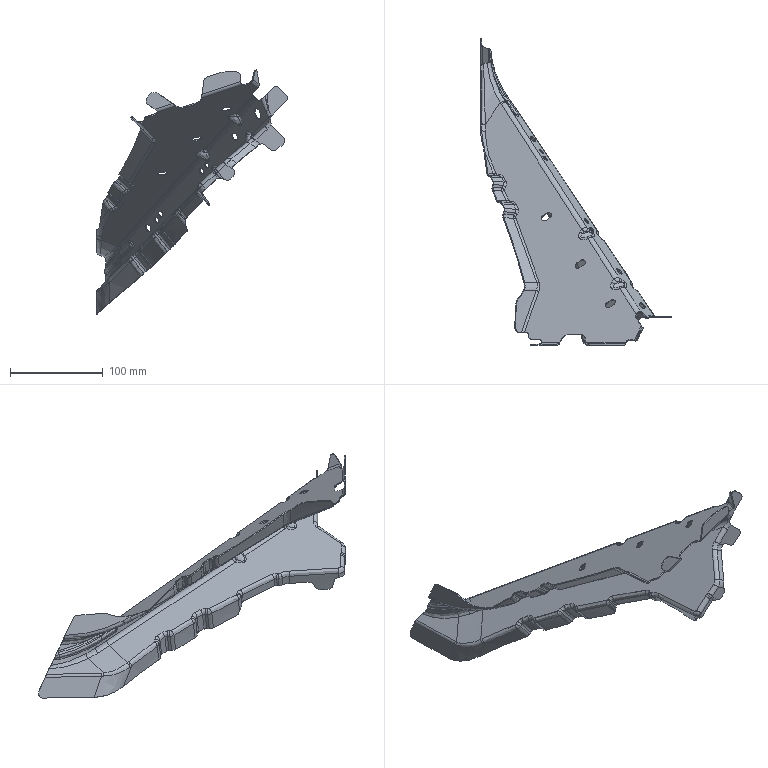Part | 1 solid | 615 faces | box 205.47 x 330.713 x 263.182 mm | volume 77521 mm3 | spline 493 | cylinder 81 | plane 33 | sphere 4 | torus 4 | commonest cylinder face diameters 6 x13 10 x12 8.4 x9 8 x8 12 x7 9.6 x6